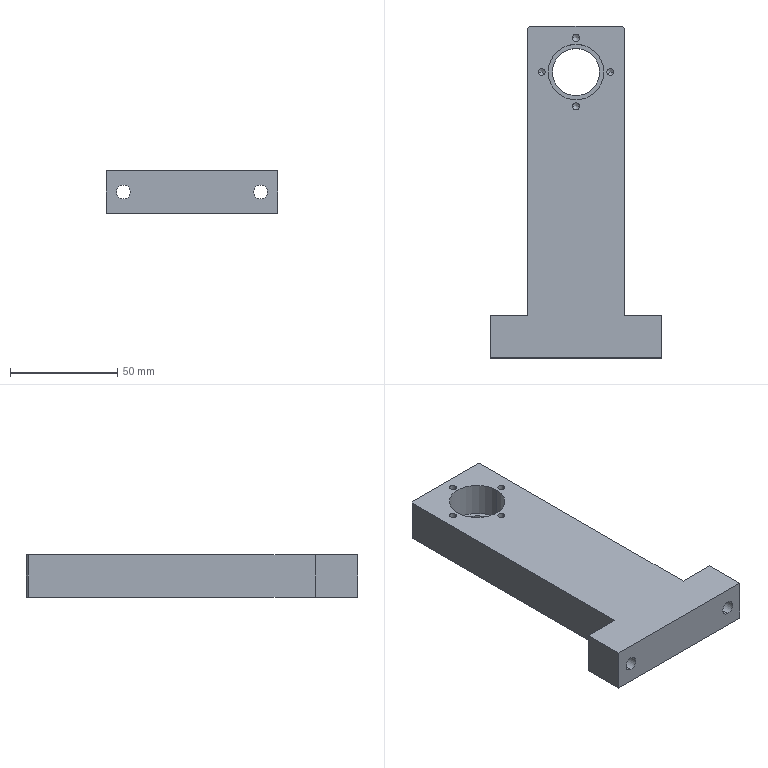Part | STEP file | PN_0093 Mount electronic clip adhesive tape support plate | 1 solid | 45 faces | box 80 x 155 x 20 mm | volume 141530 mm3 | cylinder 20 | plane 13 | cone 12 | commonest cylinder face diameters 3.3 x12 6.5 x4 22 x2 26 x2